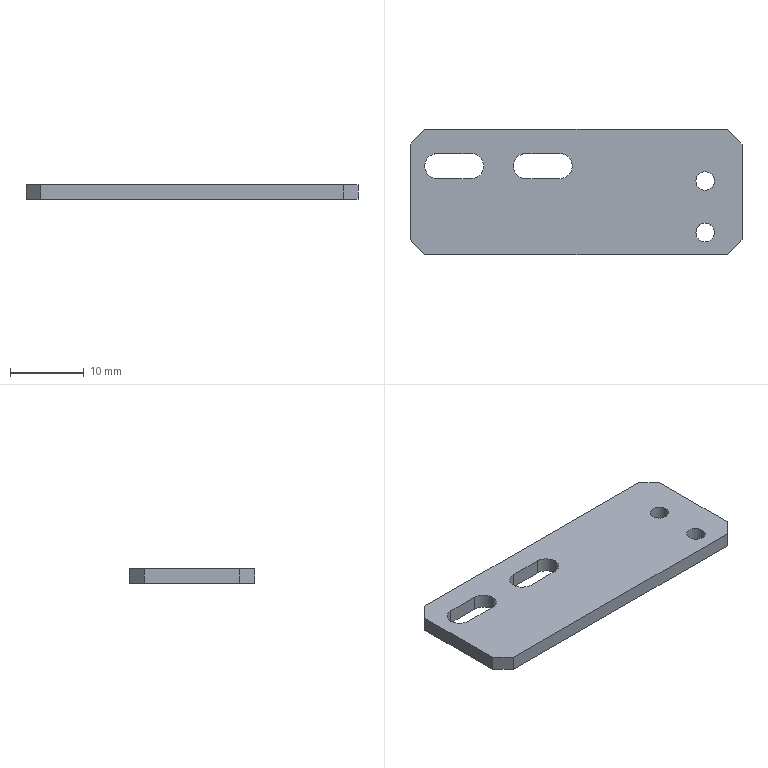Part | STEP file | FBDS-CS-006 | 1 solid | 24 faces | box 45 x 17 x 2 mm | volume 1395 mm3 | plane 14 | cylinder 10 | commonest cylinder face diameters 3.4 x6 2.5 x4
STEP:
#1=CARTESIAN_POINT('',(16.25,1.5,-2.));
#2=VERTEX_POINT('',#1);
#3=CARTESIAN_POINT('',(18.75,1.5,-2.));
#4=VERTEX_POINT('',#3);
#5=CARTESIAN_POINT('',(17.5,1.5,-2.));
#6=DIRECTION('',(0.,0.,1.));
#7=DIRECTION('',(1.,0.,0.));
#8=AXIS2_PLACEMENT_3D('',#5,#6,#7);
#9=CIRCLE('',#8,1.25);
#10=EDGE_CURVE('',#2,#4,#9,.T.);
#11=ORIENTED_EDGE('',*,*,#10,.F.);
#12=CARTESIAN_POINT('',(16.25,1.5,0.));
#13=VERTEX_POINT('',#12);
#14=CARTESIAN_POINT('',(16.25,1.5,0.));
#15=DIRECTION('',(0.,0.,1.));
#16=VECTOR('',#15,1000.);
#17=LINE('',#14,#16);
#18=EDGE_CURVE('',#2,#13,#17,.T.);
#19=ORIENTED_EDGE('',*,*,#18,.T.);
#20=CARTESIAN_POINT('',(18.75,1.5,0.));
#21=VERTEX_POINT('',#20);
#22=CARTESIAN_POINT('',(17.5,1.5,0.));
#23=DIRECTION('',(0.,0.,1.));
#24=DIRECTION('',(1.,0.,0.));
#25=AXIS2_PLACEMENT_3D('',#22,#23,#24);
#26=CIRCLE('',#25,1.25);
#27=EDGE_CURVE('',#13,#21,#26,.T.);
#28=ORIENTED_EDGE('',*,*,#27,.T.);
#29=CARTESIAN_POINT('',(18.75,1.5,0.));
#30=DIRECTION('',(0.,0.,1.));
#31=VECTOR('',#30,1000.);
#32=LINE('',#29,#31);
#33=EDGE_CURVE('',#4,#21,#32,.T.);
#34=ORIENTED_EDGE('',*,*,#33,.F.);
#35=EDGE_LOOP('',(#11,#19,#28,#34));
#36=FACE_OUTER_BOUND('',#35,.T.);
#37=CARTESIAN_POINT('',(17.5,1.5,0.));
#38=DIRECTION('',(0.,0.,1.));
#39=DIRECTION('',(1.,0.,0.));
#40=AXIS2_PLACEMENT_3D('',#37,#38,#39);
#41=CYLINDRICAL_SURFACE('',#40,1.25);
#42=ADVANCED_FACE('',(#36),#41,.F.);
#43=CARTESIAN_POINT('',(16.25,-5.5,-2.));
#44=VERTEX_POINT('',#43);
#45=CARTESIAN_POINT('',(18.75,-5.5,-2.));
#46=VERTEX_POINT('',#45);
#47=CARTESIAN_POINT('',(17.5,-5.5,-2.));
#48=DIRECTION('',(0.,0.,1.));
#49=DIRECTION('',(1.,0.,0.));
#50=AXIS2_PLACEMENT_3D('',#47,#48,#49);
#51=CIRCLE('',#50,1.25);
#52=EDGE_CURVE('',#44,#46,#51,.T.);
#53=ORIENTED_EDGE('',*,*,#52,.F.);
#54=CARTESIAN_POINT('',(16.25,-5.5,0.));
#55=VERTEX_POINT('',#54);
#56=CARTESIAN_POINT('',(16.25,-5.5,0.));
#57=DIRECTION('',(0.,0.,1.));
#58=VECTOR('',#57,1000.);
#59=LINE('',#56,#58);
#60=EDGE_CURVE('',#44,#55,#59,.T.);
#61=ORIENTED_EDGE('',*,*,#60,.T.);
#62=CARTESIAN_POINT('',(18.75,-5.5,0.));
#63=VERTEX_POINT('',#62);
#64=CARTESIAN_POINT('',(17.5,-5.5,0.));
#65=DIRECTION('',(0.,0.,1.));
#66=DIRECTION('',(1.,0.,0.));
#67=AXIS2_PLACEMENT_3D('',#64,#65,#66);
#68=CIRCLE('',#67,1.25);
#69=EDGE_CURVE('',#55,#63,#68,.T.);
#70=ORIENTED_EDGE('',*,*,#69,.T.);
#71=CARTESIAN_POINT('',(18.75,-5.5,0.));
#72=DIRECTION('',(0.,0.,1.));
#73=VECTOR('',#72,1000.);
#74=LINE('',#71,#73);
#75=EDGE_CURVE('',#46,#63,#74,.T.);
#76=ORIENTED_EDGE('',*,*,#75,.F.);
#77=EDGE_LOOP('',(#53,#61,#70,#76));
#78=FACE_OUTER_BOUND('',#77,.T.);
#79=CARTESIAN_POINT('',(17.5,-5.5,0.));
#80=DIRECTION('',(0.,0.,1.));
#81=DIRECTION('',(1.,0.,0.));
#82=AXIS2_PLACEMENT_3D('',#79,#80,#81);
#83=CYLINDRICAL_SURFACE('',#82,1.25);
#84=ADVANCED_FACE('',(#78),#83,.F.);
#85=CARTESIAN_POINT('',(-12.5,3.5,-2.));
#86=VERTEX_POINT('',#85);
#87=CARTESIAN_POINT('',(-14.2,5.2,-2.));
#88=VERTEX_POINT('',#87);
#89=CARTESIAN_POINT('',(-14.2,3.5,-2.));
#90=DIRECTION('',(0.,0.,1.));
#91=DIRECTION('',(1.,0.,0.));
#92=AXIS2_PLACEMENT_3D('',#89,#90,#91);
#93=CIRCLE('',#92,1.7);
#94=EDGE_CURVE('',#86,#88,#93,.T.);
#95=ORIENTED_EDGE('',*,*,#94,.F.);
#96=CARTESIAN_POINT('',(-12.5,3.5,0.));
#97=VERTEX_POINT('',#96);
#98=CARTESIAN_POINT('',(-12.5,3.5,0.));
#99=DIRECTION('',(0.,0.,1.));
#100=VECTOR('',#99,1000.);
#101=LINE('',#98,#100);
#102=EDGE_CURVE('',#86,#97,#101,.T.);
#103=ORIENTED_EDGE('',*,*,#102,.T.);
#104=CARTESIAN_POINT('',(-14.2,5.2,0.));
#105=VERTEX_POINT('',#104);
#106=CARTESIAN_POINT('',(-14.2,3.5,0.));
#107=DIRECTION('',(0.,0.,1.));
#108=DIRECTION('',(1.,0.,0.));
#109=AXIS2_PLACEMENT_3D('',#106,#107,#108);
#110=CIRCLE('',#109,1.7);
#111=EDGE_CURVE('',#97,#105,#110,.T.);
#112=ORIENTED_EDGE('',*,*,#111,.T.);
#113=CARTESIAN_POINT('',(-14.2,5.2,0.));
#114=DIRECTION('',(0.,0.,1.));
#115=VECTOR('',#114,1000.);
#116=LINE('',#113,#115);
#117=EDGE_CURVE('',#88,#105,#116,.T.);
#118=ORIENTED_EDGE('',*,*,#117,.F.);
#119=EDGE_LOOP('',(#95,#103,#112,#118));
#120=FACE_OUTER_BOUND('',#119,.T.);
#121=CARTESIAN_POINT('',(-14.2,3.5,0.));
#122=DIRECTION('',(0.,0.,1.));
#123=DIRECTION('',(1.,0.,0.));
#124=AXIS2_PLACEMENT_3D('',#121,#122,#123);
#125=CYLINDRICAL_SURFACE('',#124,1.7);
#126=ADVANCED_FACE('',(#120),#125,.F.);
#127=CARTESIAN_POINT('',(-0.5,3.5,-2.));
#128=VERTEX_POINT('',#127);
#129=CARTESIAN_POINT('',(-2.2,5.2,-2.));
#130=VERTEX_POINT('',#129);
#131=CARTESIAN_POINT('',(-2.2,3.5,-2.));
#132=DIRECTION('',(0.,0.,1.));
#133=DIRECTION('',(1.,0.,0.));
#134=AXIS2_PLACEMENT_3D('',#131,#132,#133);
#135=CIRCLE('',#134,1.7);
#136=EDGE_CURVE('',#128,#130,#135,.T.);
#137=ORIENTED_EDGE('',*,*,#136,.F.);
#138=CARTESIAN_POINT('',(-0.5,3.5,0.));
#139=VERTEX_POINT('',#138);
#140=CARTESIAN_POINT('',(-0.5,3.5,0.));
#141=DIRECTION('',(0.,0.,1.));
#142=VECTOR('',#141,1000.);
#143=LINE('',#140,#142);
#144=EDGE_CURVE('',#128,#139,#143,.T.);
#145=ORIENTED_EDGE('',*,*,#144,.T.);
#146=CARTESIAN_POINT('',(-2.2,5.2,0.));
#147=VERTEX_POINT('',#146);
#148=CARTESIAN_POINT('',(-2.2,3.5,0.));
#149=DIRECTION('',(0.,0.,1.));
#150=DIRECTION('',(1.,0.,0.));
#151=AXIS2_PLACEMENT_3D('',#148,#149,#150);
#152=CIRCLE('',#151,1.7);
#153=EDGE_CURVE('',#139,#147,#152,.T.);
#154=ORIENTED_EDGE('',*,*,#153,.T.);
#155=CARTESIAN_POINT('',(-2.2,5.2,0.));
#156=DIRECTION('',(0.,0.,1.));
#157=VECTOR('',#156,1000.);
#158=LINE('',#155,#157);
#159=EDGE_CURVE('',#130,#147,#158,.T.);
#160=ORIENTED_EDGE('',*,*,#159,.F.);
#161=EDGE_LOOP('',(#137,#145,#154,#160));
#162=FACE_OUTER_BOUND('',#161,.T.);
#163=CARTESIAN_POINT('',(-2.2,3.5,0.));
#164=DIRECTION('',(0.,0.,1.));
#165=DIRECTION('',(1.,0.,0.));
#166=AXIS2_PLACEMENT_3D('',#163,#164,#165);
#167=CYLINDRICAL_SURFACE('',#166,1.7);
#168=ADVANCED_FACE('',(#162),#167,.F.);
#169=CARTESIAN_POINT('',(22.5,-6.5,-2.));
#170=VERTEX_POINT('',#169);
#171=CARTESIAN_POINT('',(22.5,6.5,-2.));
#172=VERTEX_POINT('',#171);
#173=CARTESIAN_POINT('',(22.5,8.5,-2.));
#174=DIRECTION('',(0.,1.,0.));
#175=VECTOR('',#174,1000.);
#176=LINE('',#173,#175);
#177=EDGE_CURVE('',#170,#172,#176,.T.);
#178=ORIENTED_EDGE('',*,*,#177,.T.);
#179=CARTESIAN_POINT('',(22.5,6.5,0.));
#180=VERTEX_POINT('',#179);
#181=CARTESIAN_POINT('',(22.5,6.5,-2.));
#182=DIRECTION('',(0.,0.,1.));
#183=VECTOR('',#182,1000.);
#184=LINE('',#181,#183);
#185=EDGE_CURVE('',#172,#180,#184,.T.);
#186=ORIENTED_EDGE('',*,*,#185,.T.);
#187=CARTESIAN_POINT('',(22.5,-6.5,0.));
#188=VERTEX_POINT('',#187);
#189=CARTESIAN_POINT('',(22.5,8.5,0.));
#190=DIRECTION('',(0.,1.,0.));
#191=VECTOR('',#190,1000.);
#192=LINE('',#189,#191);
#193=EDGE_CURVE('',#188,#180,#192,.T.);
#194=ORIENTED_EDGE('',*,*,#193,.F.);
#195=CARTESIAN_POINT('',(22.5,-6.5,-2.));
#196=DIRECTION('',(0.,0.,-1.));
#197=VECTOR('',#196,1000.);
#198=LINE('',#195,#197);
#199=EDGE_CURVE('',#188,#170,#198,.T.);
#200=ORIENTED_EDGE('',*,*,#199,.T.);
#201=EDGE_LOOP('',(#178,#186,#194,#200));
#202=FACE_OUTER_BOUND('',#201,.T.);
#203=CARTESIAN_POINT('',(22.5,8.5,-2.));
#204=DIRECTION('',(1.,0.,0.));
#205=DIRECTION('',(0.,0.,-1.));
#206=AXIS2_PLACEMENT_3D('',#203,#204,#205);
#207=PLANE('',#206);
#208=ADVANCED_FACE('',(#202),#207,.T.);
#209=CARTESIAN_POINT('',(-20.5,-8.5,-2.));
#210=VERTEX_POINT('',#209);
#211=CARTESIAN_POINT('',(20.5,-8.5,-2.));
#212=VERTEX_POINT('',#211);
#213=CARTESIAN_POINT('',(-22.5,-8.5,-2.));
#214=DIRECTION('',(1.,0.,0.));
#215=VECTOR('',#214,1000.);
#216=LINE('',#213,#215);
#217=EDGE_CURVE('',#210,#212,#216,.T.);
#218=ORIENTED_EDGE('',*,*,#217,.T.);
#219=CARTESIAN_POINT('',(20.5,-8.5,0.));
#220=VERTEX_POINT('',#219);
#221=CARTESIAN_POINT('',(20.5,-8.5,-2.));
#222=DIRECTION('',(0.,0.,1.));
#223=VECTOR('',#222,1000.);
#224=LINE('',#221,#223);
#225=EDGE_CURVE('',#212,#220,#224,.T.);
#226=ORIENTED_EDGE('',*,*,#225,.T.);
#227=CARTESIAN_POINT('',(-20.5,-8.5,0.));
#228=VERTEX_POINT('',#227);
#229=CARTESIAN_POINT('',(-22.5,-8.5,0.));
#230=DIRECTION('',(1.,0.,0.));
#231=VECTOR('',#230,1000.);
#232=LINE('',#229,#231);
#233=EDGE_CURVE('',#228,#220,#232,.T.);
#234=ORIENTED_EDGE('',*,*,#233,.F.);
#235=CARTESIAN_POINT('',(-20.5,-8.5,-2.));
#236=DIRECTION('',(0.,0.,-1.));
#237=VECTOR('',#236,1000.);
#238=LINE('',#235,#237);
#239=EDGE_CURVE('',#228,#210,#238,.T.);
#240=ORIENTED_EDGE('',*,*,#239,.T.);
#241=EDGE_LOOP('',(#218,#226,#234,#240));
#242=FACE_OUTER_BOUND('',#241,.T.);
#243=CARTESIAN_POINT('',(-22.5,-8.5,-2.));
#244=DIRECTION('',(0.,-1.,0.));
#245=DIRECTION('',(0.,0.,-1.));
#246=AXIS2_PLACEMENT_3D('',#243,#244,#245);
#247=PLANE('',#246);
#248=ADVANCED_FACE('',(#242),#247,.T.);
#249=CARTESIAN_POINT('',(-22.5,6.5,-2.));
#250=VERTEX_POINT('',#249);
#251=CARTESIAN_POINT('',(-22.5,-6.5,-2.));
#252=VERTEX_POINT('',#251);
#253=CARTESIAN_POINT('',(-22.5,8.5,-2.));
#254=DIRECTION('',(0.,-1.,0.));
#255=VECTOR('',#254,1000.);
#256=LINE('',#253,#255);
#257=EDGE_CURVE('',#250,#252,#256,.T.);
#258=ORIENTED_EDGE('',*,*,#257,.T.);
#259=CARTESIAN_POINT('',(-22.5,-6.5,0.));
#260=VERTEX_POINT('',#259);
#261=CARTESIAN_POINT('',(-22.5,-6.5,-2.));
#262=DIRECTION('',(0.,0.,1.));
#263=VECTOR('',#262,1000.);
#264=LINE('',#261,#263);
#265=EDGE_CURVE('',#252,#260,#264,.T.);
#266=ORIENTED_EDGE('',*,*,#265,.T.);
#267=CARTESIAN_POINT('',(-22.5,6.5,0.));
#268=VERTEX_POINT('',#267);
#269=CARTESIAN_POINT('',(-22.5,8.5,0.));
#270=DIRECTION('',(0.,-1.,0.));
#271=VECTOR('',#270,1000.);
#272=LINE('',#269,#271);
#273=EDGE_CURVE('',#268,#260,#272,.T.);
#274=ORIENTED_EDGE('',*,*,#273,.F.);
#275=CARTESIAN_POINT('',(-22.5,6.5,-2.));
#276=DIRECTION('',(0.,0.,-1.));
#277=VECTOR('',#276,1000.);
#278=LINE('',#275,#277);
#279=EDGE_CURVE('',#268,#250,#278,.T.);
#280=ORIENTED_EDGE('',*,*,#279,.T.);
#281=EDGE_LOOP('',(#258,#266,#274,#280));
#282=FACE_OUTER_BOUND('',#281,.T.);
#283=CARTESIAN_POINT('',(-22.5,8.5,-2.));
#284=DIRECTION('',(-1.,0.,0.));
#285=DIRECTION('',(0.,-1.,0.));
#286=AXIS2_PLACEMENT_3D('',#283,#284,#285);
#287=PLANE('',#286);
#288=ADVANCED_FACE('',(#282),#287,.T.);
#289=CARTESIAN_POINT('',(20.5,8.5,0.));
#290=VERTEX_POINT('',#289);
#291=CARTESIAN_POINT('',(-20.5,8.5,0.));
#292=VERTEX_POINT('',#291);
#293=CARTESIAN_POINT('',(-22.5,8.5,0.));
#294=DIRECTION('',(-1.,0.,0.));
#295=VECTOR('',#294,1000.);
#296=LINE('',#293,#295);
#297=EDGE_CURVE('',#290,#292,#296,.T.);
#298=ORIENTED_EDGE('',*,*,#297,.F.);
#299=CARTESIAN_POINT('',(20.5,8.5,-2.));
#300=VERTEX_POINT('',#299);
#301=CARTESIAN_POINT('',(20.5,8.5,-2.));
#302=DIRECTION('',(0.,0.,-1.));
#303=VECTOR('',#302,1000.);
#304=LINE('',#301,#303);
#305=EDGE_CURVE('',#290,#300,#304,.T.);
#306=ORIENTED_EDGE('',*,*,#305,.T.);
#307=CARTESIAN_POINT('',(-20.5,8.5,-2.));
#308=VERTEX_POINT('',#307);
#309=CARTESIAN_POINT('',(-22.5,8.5,-2.));
#310=DIRECTION('',(-1.,0.,0.));
#311=VECTOR('',#310,1000.);
#312=LINE('',#309,#311);
#313=EDGE_CURVE('',#300,#308,#312,.T.);
#314=ORIENTED_EDGE('',*,*,#313,.T.);
#315=CARTESIAN_POINT('',(-20.5,8.5,-2.));
#316=DIRECTION('',(0.,0.,1.));
#317=VECTOR('',#316,1000.);
#318=LINE('',#315,#317);
#319=EDGE_CURVE('',#308,#292,#318,.T.);
#320=ORIENTED_EDGE('',*,*,#319,.T.);
#321=EDGE_LOOP('',(#298,#306,#314,#320));
#322=FACE_OUTER_BOUND('',#321,.T.);
#323=CARTESIAN_POINT('',(-22.5,8.5,-2.));
#324=DIRECTION('',(0.,1.,0.));
#325=DIRECTION('',(0.,0.,1.));
#326=AXIS2_PLACEMENT_3D('',#323,#324,#325);
#327=PLANE('',#326);
#328=ADVANCED_FACE('',(#322),#327,.T.);
#329=CARTESIAN_POINT('',(17.5,1.5,-2.));
#330=DIRECTION('',(0.,0.,1.));
#331=DIRECTION('',(1.,0.,0.));
#332=AXIS2_PLACEMENT_3D('',#329,#330,#331);
#333=CIRCLE('',#332,1.25);
#334=EDGE_CURVE('',#4,#2,#333,.T.);
#335=ORIENTED_EDGE('',*,*,#334,.T.);
#336=ORIENTED_EDGE('',*,*,#10,.T.);
#337=EDGE_LOOP('',(#335,#336));
#338=FACE_BOUND('',#337,.T.);
#339=CARTESIAN_POINT('',(17.5,-5.5,-2.));
#340=DIRECTION('',(0.,0.,1.));
#341=DIRECTION('',(1.,0.,0.));
#342=AXIS2_PLACEMENT_3D('',#339,#340,#341);
#343=CIRCLE('',#342,1.25);
#344=EDGE_CURVE('',#46,#44,#343,.T.);
#345=ORIENTED_EDGE('',*,*,#344,.T.);
#346=ORIENTED_EDGE('',*,*,#52,.T.);
#347=EDGE_LOOP('',(#345,#346));
#348=FACE_BOUND('',#347,.T.);
#349=CARTESIAN_POINT('',(-14.2,1.8,-2.));
#350=VERTEX_POINT('',#349);
#351=CARTESIAN_POINT('',(-14.2,3.5,-2.));
#352=DIRECTION('',(0.,0.,1.));
#353=DIRECTION('',(1.,0.,0.));
#354=AXIS2_PLACEMENT_3D('',#351,#352,#353);
#355=CIRCLE('',#354,1.7);
#356=EDGE_CURVE('',#350,#86,#355,.T.);
#357=ORIENTED_EDGE('',*,*,#356,.T.);
#358=ORIENTED_EDGE('',*,*,#94,.T.);
#359=CARTESIAN_POINT('',(-18.8,5.2,-2.));
#360=VERTEX_POINT('',#359);
#361=CARTESIAN_POINT('',(0.,5.2,-2.));
#362=DIRECTION('',(-1.,0.,0.));
#363=VECTOR('',#362,1000.);
#364=LINE('',#361,#363);
#365=EDGE_CURVE('',#88,#360,#364,.T.);
#366=ORIENTED_EDGE('',*,*,#365,.T.);
#367=CARTESIAN_POINT('',(-18.8,1.8,-2.));
#368=VERTEX_POINT('',#367);
#369=CARTESIAN_POINT('',(-18.8,3.5,-2.));
#370=DIRECTION('',(0.,0.,1.));
#371=DIRECTION('',(1.,0.,0.));
#372=AXIS2_PLACEMENT_3D('',#369,#370,#371);
#373=CIRCLE('',#372,1.7);
#374=EDGE_CURVE('',#360,#368,#373,.T.);
#375=ORIENTED_EDGE('',*,*,#374,.T.);
#376=CARTESIAN_POINT('',(0.,1.8,-2.));
#377=DIRECTION('',(1.,0.,0.));
#378=VECTOR('',#377,1000.);
#379=LINE('',#376,#378);
#380=EDGE_CURVE('',#368,#350,#379,.T.);
#381=ORIENTED_EDGE('',*,*,#380,.T.);
#382=EDGE_LOOP('',(#357,#358,#366,#375,#381));
#383=FACE_BOUND('',#382,.T.);
#384=CARTESIAN_POINT('',(-6.8,1.8,-2.));
#385=VERTEX_POINT('',#384);
#386=CARTESIAN_POINT('',(-2.2,1.8,-2.));
#387=VERTEX_POINT('',#386);
#388=CARTESIAN_POINT('',(0.,1.8,-2.));
#389=DIRECTION('',(1.,0.,0.));
#390=VECTOR('',#389,1000.);
#391=LINE('',#388,#390);
#392=EDGE_CURVE('',#385,#387,#391,.T.);
#393=ORIENTED_EDGE('',*,*,#392,.T.);
#394=CARTESIAN_POINT('',(-2.2,3.5,-2.));
#395=DIRECTION('',(0.,0.,1.));
#396=DIRECTION('',(1.,0.,0.));
#397=AXIS2_PLACEMENT_3D('',#394,#395,#396);
#398=CIRCLE('',#397,1.7);
#399=EDGE_CURVE('',#387,#128,#398,.T.);
#400=ORIENTED_EDGE('',*,*,#399,.T.);
#401=ORIENTED_EDGE('',*,*,#136,.T.);
#402=CARTESIAN_POINT('',(-6.8,5.2,-2.));
#403=VERTEX_POINT('',#402);
#404=CARTESIAN_POINT('',(0.,5.2,-2.));
#405=DIRECTION('',(-1.,0.,0.));
#406=VECTOR('',#405,1000.);
#407=LINE('',#404,#406);
#408=EDGE_CURVE('',#130,#403,#407,.T.);
#409=ORIENTED_EDGE('',*,*,#408,.T.);
#410=CARTESIAN_POINT('',(-6.8,3.5,-2.));
#411=DIRECTION('',(0.,0.,1.));
#412=DIRECTION('',(1.,0.,0.));
#413=AXIS2_PLACEMENT_3D('',#410,#411,#412);
#414=CIRCLE('',#413,1.7);
#415=EDGE_CURVE('',#403,#385,#414,.T.);
#416=ORIENTED_EDGE('',*,*,#415,.T.);
#417=EDGE_LOOP('',(#393,#400,#401,#409,#416));
#418=FACE_BOUND('',#417,.T.);
#419=ORIENTED_EDGE('',*,*,#313,.F.);
#420=CARTESIAN_POINT('',(22.5,6.5,-2.));
#421=DIRECTION('',(0.7071,-0.7071,0.));
#422=VECTOR('',#421,1000.);
#423=LINE('',#420,#422);
#424=EDGE_CURVE('',#300,#172,#423,.T.);
#425=ORIENTED_EDGE('',*,*,#424,.T.);
#426=ORIENTED_EDGE('',*,*,#177,.F.);
#427=CARTESIAN_POINT('',(20.5,-8.5,-2.));
#428=DIRECTION('',(-0.7071,-0.7071,0.));
#429=VECTOR('',#428,1000.);
#430=LINE('',#427,#429);
#431=EDGE_CURVE('',#170,#212,#430,.T.);
#432=ORIENTED_EDGE('',*,*,#431,.T.);
#433=ORIENTED_EDGE('',*,*,#217,.F.);
#434=CARTESIAN_POINT('',(-22.5,-6.5,-2.));
#435=DIRECTION('',(-0.7071,0.7071,0.));
#436=VECTOR('',#435,1000.);
#437=LINE('',#434,#436);
#438=EDGE_CURVE('',#210,#252,#437,.T.);
#439=ORIENTED_EDGE('',*,*,#438,.T.);
#440=ORIENTED_EDGE('',*,*,#257,.F.);
#441=CARTESIAN_POINT('',(-20.5,8.5,-2.));
#442=DIRECTION('',(0.7071,0.7071,0.));
#443=VECTOR('',#442,1000.);
#444=LINE('',#441,#443);
#445=EDGE_CURVE('',#250,#308,#444,.T.);
#446=ORIENTED_EDGE('',*,*,#445,.T.);
#447=EDGE_LOOP('',(#419,#425,#426,#432,#433,#439,#440,#446));
#448=FACE_OUTER_BOUND('',#447,.T.);
#449=CARTESIAN_POINT('',(0.,0.,-2.));
#450=DIRECTION('',(0.,0.,1.));
#451=DIRECTION('',(1.,0.,0.));
#452=AXIS2_PLACEMENT_3D('',#449,#450,#451);
#453=PLANE('',#452);
#454=ADVANCED_FACE('',(#338,#348,#383,#418,#448),#453,.F.);
#455=CARTESIAN_POINT('',(17.5,1.5,0.));
#456=DIRECTION('',(0.,0.,1.));
#457=DIRECTION('',(1.,0.,0.));
#458=AXIS2_PLACEMENT_3D('',#455,#456,#457);
#459=CIRCLE('',#458,1.25);
#460=EDGE_CURVE('',#21,#13,#459,.T.);
#461=ORIENTED_EDGE('',*,*,#460,.F.);
#462=ORIENTED_EDGE('',*,*,#27,.F.);
#463=EDGE_LOOP('',(#461,#462));
#464=FACE_BOUND('',#463,.T.);
#465=CARTESIAN_POINT('',(17.5,-5.5,0.));
#466=DIRECTION('',(0.,0.,1.));
#467=DIRECTION('',(1.,0.,0.));
#468=AXIS2_PLACEMENT_3D('',#465,#466,#467);
#469=CIRCLE('',#468,1.25);
#470=EDGE_CURVE('',#63,#55,#469,.T.);
#471=ORIENTED_EDGE('',*,*,#470,.F.);
#472=ORIENTED_EDGE('',*,*,#69,.F.);
#473=EDGE_LOOP('',(#471,#472));
#474=FACE_BOUND('',#473,.T.);
#475=CARTESIAN_POINT('',(-18.8,1.8,0.));
#476=VERTEX_POINT('',#475);
#477=CARTESIAN_POINT('',(-14.2,1.8,0.));
#478=VERTEX_POINT('',#477);
#479=CARTESIAN_POINT('',(-18.8,1.8,0.));
#480=DIRECTION('',(1.,0.,0.));
#481=VECTOR('',#480,1000.);
#482=LINE('',#479,#481);
#483=EDGE_CURVE('',#476,#478,#482,.T.);
#484=ORIENTED_EDGE('',*,*,#483,.F.);
#485=CARTESIAN_POINT('',(-18.8,5.2,0.));
#486=VERTEX_POINT('',#485);
#487=CARTESIAN_POINT('',(-18.8,3.5,0.));
#488=DIRECTION('',(0.,0.,1.));
#489=DIRECTION('',(1.,0.,0.));
#490=AXIS2_PLACEMENT_3D('',#487,#488,#489);
#491=CIRCLE('',#490,1.7);
#492=EDGE_CURVE('',#486,#476,#491,.T.);
#493=ORIENTED_EDGE('',*,*,#492,.F.);
#494=CARTESIAN_POINT('',(-18.8,5.2,0.));
#495=DIRECTION('',(1.,0.,0.));
#496=VECTOR('',#495,1000.);
#497=LINE('',#494,#496);
#498=EDGE_CURVE('',#486,#105,#497,.T.);
#499=ORIENTED_EDGE('',*,*,#498,.T.);
#500=ORIENTED_EDGE('',*,*,#111,.F.);
#501=CARTESIAN_POINT('',(-14.2,3.5,0.));
#502=DIRECTION('',(0.,0.,1.));
#503=DIRECTION('',(1.,0.,0.));
#504=AXIS2_PLACEMENT_3D('',#501,#502,#503);
#505=CIRCLE('',#504,1.7);
#506=EDGE_CURVE('',#478,#97,#505,.T.);
#507=ORIENTED_EDGE('',*,*,#506,.F.);
#508=EDGE_LOOP('',(#484,#493,#499,#500,#507));
#509=FACE_BOUND('',#508,.T.);
#510=CARTESIAN_POINT('',(-6.8,1.8,0.));
#511=VERTEX_POINT('',#510);
#512=CARTESIAN_POINT('',(-2.2,1.8,0.));
#513=VERTEX_POINT('',#512);
#514=CARTESIAN_POINT('',(-6.8,1.8,0.));
#515=DIRECTION('',(1.,0.,0.));
#516=VECTOR('',#515,1000.);
#517=LINE('',#514,#516);
#518=EDGE_CURVE('',#511,#513,#517,.T.);
#519=ORIENTED_EDGE('',*,*,#518,.F.);
#520=CARTESIAN_POINT('',(-6.8,5.2,0.));
#521=VERTEX_POINT('',#520);
#522=CARTESIAN_POINT('',(-6.8,3.5,0.));
#523=DIRECTION('',(0.,0.,1.));
#524=DIRECTION('',(1.,0.,0.));
#525=AXIS2_PLACEMENT_3D('',#522,#523,#524);
#526=CIRCLE('',#525,1.7);
#527=EDGE_CURVE('',#521,#511,#526,.T.);
#528=ORIENTED_EDGE('',*,*,#527,.F.);
#529=CARTESIAN_POINT('',(-6.8,5.2,0.));
#530=DIRECTION('',(1.,0.,0.));
#531=VECTOR('',#530,1000.);
#532=LINE('',#529,#531);
#533=EDGE_CURVE('',#521,#147,#532,.T.);
#534=ORIENTED_EDGE('',*,*,#533,.T.);
#535=ORIENTED_EDGE('',*,*,#153,.F.);
#536=CARTESIAN_POINT('',(-2.2,3.5,0.));
#537=DIRECTION('',(0.,0.,1.));
#538=DIRECTION('',(1.,0.,0.));
#539=AXIS2_PLACEMENT_3D('',#536,#537,#538);
#540=CIRCLE('',#539,1.7);
#541=EDGE_CURVE('',#513,#139,#540,.T.);
#542=ORIENTED_EDGE('',*,*,#541,.F.);
#543=EDGE_LOOP('',(#519,#528,#534,#535,#542));
#544=FACE_BOUND('',#543,.T.);
#545=ORIENTED_EDGE('',*,*,#193,.T.);
#546=CARTESIAN_POINT('',(14.5,14.5,0.));
#547=DIRECTION('',(-0.7071,0.7071,0.));
#548=VECTOR('',#547,1000.);
#549=LINE('',#546,#548);
#550=EDGE_CURVE('',#180,#290,#549,.T.);
#551=ORIENTED_EDGE('',*,*,#550,.T.);
#552=ORIENTED_EDGE('',*,*,#297,.T.);
#553=CARTESIAN_POINT('',(-14.5,14.5,0.));
#554=DIRECTION('',(-0.7071,-0.7071,0.));
#555=VECTOR('',#554,1000.);
#556=LINE('',#553,#555);
#557=EDGE_CURVE('',#292,#268,#556,.T.);
#558=ORIENTED_EDGE('',*,*,#557,.T.);
#559=ORIENTED_EDGE('',*,*,#273,.T.);
#560=CARTESIAN_POINT('',(-14.5,-14.5,0.));
#561=DIRECTION('',(0.7071,-0.7071,0.));
#562=VECTOR('',#561,1000.);
#563=LINE('',#560,#562);
#564=EDGE_CURVE('',#260,#228,#563,.T.);
#565=ORIENTED_EDGE('',*,*,#564,.T.);
#566=ORIENTED_EDGE('',*,*,#233,.T.);
#567=CARTESIAN_POINT('',(14.5,-14.5,0.));
#568=DIRECTION('',(0.7071,0.7071,0.));
#569=VECTOR('',#568,1000.);
#570=LINE('',#567,#569);
#571=EDGE_CURVE('',#220,#188,#570,.T.);
#572=ORIENTED_EDGE('',*,*,#571,.T.);
#573=EDGE_LOOP('',(#545,#551,#552,#558,#559,#565,#566,#572));
#574=FACE_OUTER_BOUND('',#573,.T.);
#575=CARTESIAN_POINT('',(0.,0.,0.));
#576=DIRECTION('',(0.,0.,1.));
#577=DIRECTION('',(1.,0.,0.));
#578=AXIS2_PLACEMENT_3D('',#575,#576,#577);
#579=PLANE('',#578);
#580=ADVANCED_FACE('',(#464,#474,#509,#544,#574),#579,.T.);
#581=CARTESIAN_POINT('',(-6.8,1.8,0.));
#582=DIRECTION('',(0.,0.,1.));
#583=VECTOR('',#582,1000.);
#584=LINE('',#581,#583);
#585=EDGE_CURVE('',#385,#511,#584,.T.);
#586=ORIENTED_EDGE('',*,*,#585,.T.);
#587=ORIENTED_EDGE('',*,*,#518,.T.);
#588=CARTESIAN_POINT('',(-2.2,1.8,0.));
#589=DIRECTION('',(0.,0.,-1.));
#590=VECTOR('',#589,1000.);
#591=LINE('',#588,#590);
#592=EDGE_CURVE('',#513,#387,#591,.T.);
#593=ORIENTED_EDGE('',*,*,#592,.T.);
#594=ORIENTED_EDGE('',*,*,#392,.F.);
#595=EDGE_LOOP('',(#586,#587,#593,#594));
#596=FACE_OUTER_BOUND('',#595,.T.);
#597=CARTESIAN_POINT('',(-6.8,1.8,0.));
#598=DIRECTION('',(0.,-1.,0.));
#599=DIRECTION('',(1.,0.,0.));
#600=AXIS2_PLACEMENT_3D('',#597,#598,#599);
#601=PLANE('',#600);
#602=ADVANCED_FACE('',(#596),#601,.F.);
#603=ORIENTED_EDGE('',*,*,#159,.T.);
#604=ORIENTED_EDGE('',*,*,#533,.F.);
#605=CARTESIAN_POINT('',(-6.8,5.2,0.));
#606=DIRECTION('',(0.,0.,-1.));
#607=VECTOR('',#606,1000.);
#608=LINE('',#605,#607);
#609=EDGE_CURVE('',#521,#403,#608,.T.);
#610=ORIENTED_EDGE('',*,*,#609,.T.);
#611=ORIENTED_EDGE('',*,*,#408,.F.);
#612=EDGE_LOOP('',(#603,#604,#610,#611));
#613=FACE_OUTER_BOUND('',#612,.T.);
#614=CARTESIAN_POINT('',(-6.8,5.2,0.));
#615=DIRECTION('',(0.,1.,0.));
#616=DIRECTION('',(-1.,0.,0.));
#617=AXIS2_PLACEMENT_3D('',#614,#615,#616);
#618=PLANE('',#617);
#619=ADVANCED_FACE('',(#613),#618,.F.);
#620=ORIENTED_EDGE('',*,*,#144,.F.);
#621=ORIENTED_EDGE('',*,*,#399,.F.);
#622=ORIENTED_EDGE('',*,*,#592,.F.);
#623=ORIENTED_EDGE('',*,*,#541,.T.);
#624=EDGE_LOOP('',(#620,#621,#622,#623));
#625=FACE_OUTER_BOUND('',#624,.T.);
#626=CARTESIAN_POINT('',(-2.2,3.5,0.));
#627=DIRECTION('',(0.,0.,1.));
#628=DIRECTION('',(1.,0.,0.));
#629=AXIS2_PLACEMENT_3D('',#626,#627,#628);
#630=CYLINDRICAL_SURFACE('',#629,1.7);
#631=ADVANCED_FACE('',(#625),#630,.F.);
#632=ORIENTED_EDGE('',*,*,#609,.F.);
#633=ORIENTED_EDGE('',*,*,#527,.T.);
#634=ORIENTED_EDGE('',*,*,#585,.F.);
#635=ORIENTED_EDGE('',*,*,#415,.F.);
#636=EDGE_LOOP('',(#632,#633,#634,#635));
#637=FACE_OUTER_BOUND('',#636,.T.);
#638=CARTESIAN_POINT('',(-6.8,3.5,0.));
#639=DIRECTION('',(0.,0.,1.));
#640=DIRECTION('',(1.,0.,0.));
#641=AXIS2_PLACEMENT_3D('',#638,#639,#640);
#642=CYLINDRICAL_SURFACE('',#641,1.7);
#643=ADVANCED_FACE('',(#637),#642,.F.);
#644=CARTESIAN_POINT('',(-18.8,5.2,0.));
#645=DIRECTION('',(0.,0.,-1.));
#646=VECTOR('',#645,1000.);
#647=LINE('',#644,#646);
#648=EDGE_CURVE('',#486,#360,#647,.T.);
#649=ORIENTED_EDGE('',*,*,#648,.F.);
#650=ORIENTED_EDGE('',*,*,#492,.T.);
#651=CARTESIAN_POINT('',(-18.8,1.8,0.));
#652=DIRECTION('',(0.,0.,1.));
#653=VECTOR('',#652,1000.);
#654=LINE('',#651,#653);
#655=EDGE_CURVE('',#368,#476,#654,.T.);
#656=ORIENTED_EDGE('',*,*,#655,.F.);
#657=ORIENTED_EDGE('',*,*,#374,.F.);
#658=EDGE_LOOP('',(#649,#650,#656,#657));
#659=FACE_OUTER_BOUND('',#658,.T.);
#660=CARTESIAN_POINT('',(-18.8,3.5,0.));
#661=DIRECTION('',(0.,0.,1.));
#662=DIRECTION('',(1.,0.,0.));
#663=AXIS2_PLACEMENT_3D('',#660,#661,#662);
#664=CYLINDRICAL_SURFACE('',#663,1.7);
#665=ADVANCED_FACE('',(#659),#664,.F.);
#666=ORIENTED_EDGE('',*,*,#117,.T.);
#667=ORIENTED_EDGE('',*,*,#498,.F.);
#668=ORIENTED_EDGE('',*,*,#648,.T.);
#669=ORIENTED_EDGE('',*,*,#365,.F.);
#670=EDGE_LOOP('',(#666,#667,#668,#669));
#671=FACE_OUTER_BOUND('',#670,.T.);
#672=CARTESIAN_POINT('',(-18.8,5.2,0.));
#673=DIRECTION('',(0.,1.,0.));
#674=DIRECTION('',(-1.,0.,0.));
#675=AXIS2_PLACEMENT_3D('',#672,#673,#674);
#676=PLANE('',#675);
#677=ADVANCED_FACE('',(#671),#676,.F.);
#678=ORIENTED_EDGE('',*,*,#655,.T.);
#679=ORIENTED_EDGE('',*,*,#483,.T.);
#680=CARTESIAN_POINT('',(-14.2,1.8,0.));
#681=DIRECTION('',(0.,0.,-1.));
#682=VECTOR('',#681,1000.);
#683=LINE('',#680,#682);
#684=EDGE_CURVE('',#478,#350,#683,.T.);
#685=ORIENTED_EDGE('',*,*,#684,.T.);
#686=ORIENTED_EDGE('',*,*,#380,.F.);
#687=EDGE_LOOP('',(#678,#679,#685,#686));
#688=FACE_OUTER_BOUND('',#687,.T.);
#689=CARTESIAN_POINT('',(-18.8,1.8,0.));
#690=DIRECTION('',(0.,-1.,0.));
#691=DIRECTION('',(1.,0.,0.));
#692=AXIS2_PLACEMENT_3D('',#689,#690,#691);
#693=PLANE('',#692);
#694=ADVANCED_FACE('',(#688),#693,.F.);
#695=ORIENTED_EDGE('',*,*,#102,.F.);
#696=ORIENTED_EDGE('',*,*,#356,.F.);
#697=ORIENTED_EDGE('',*,*,#684,.F.);
#698=ORIENTED_EDGE('',*,*,#506,.T.);
#699=EDGE_LOOP('',(#695,#696,#697,#698));
#700=FACE_OUTER_BOUND('',#699,.T.);
#701=CARTESIAN_POINT('',(-14.2,3.5,0.));
#702=DIRECTION('',(0.,0.,1.));
#703=DIRECTION('',(1.,0.,0.));
#704=AXIS2_PLACEMENT_3D('',#701,#702,#703);
#705=CYLINDRICAL_SURFACE('',#704,1.7);
#706=ADVANCED_FACE('',(#700),#705,.F.);
#707=ORIENTED_EDGE('',*,*,#60,.F.);
#708=ORIENTED_EDGE('',*,*,#344,.F.);
#709=ORIENTED_EDGE('',*,*,#75,.T.);
#710=ORIENTED_EDGE('',*,*,#470,.T.);
#711=EDGE_LOOP('',(#707,#708,#709,#710));
#712=FACE_OUTER_BOUND('',#711,.T.);
#713=CARTESIAN_POINT('',(17.5,-5.5,0.));
#714=DIRECTION('',(0.,0.,1.));
#715=DIRECTION('',(1.,0.,0.));
#716=AXIS2_PLACEMENT_3D('',#713,#714,#715);
#717=CYLINDRICAL_SURFACE('',#716,1.25);
#718=ADVANCED_FACE('',(#712),#717,.F.);
#719=ORIENTED_EDGE('',*,*,#18,.F.);
#720=ORIENTED_EDGE('',*,*,#334,.F.);
#721=ORIENTED_EDGE('',*,*,#33,.T.);
#722=ORIENTED_EDGE('',*,*,#460,.T.);
#723=EDGE_LOOP('',(#719,#720,#721,#722));
#724=FACE_OUTER_BOUND('',#723,.T.);
#725=CARTESIAN_POINT('',(17.5,1.5,0.));
#726=DIRECTION('',(0.,0.,1.));
#727=DIRECTION('',(1.,0.,0.));
#728=AXIS2_PLACEMENT_3D('',#725,#726,#727);
#729=CYLINDRICAL_SURFACE('',#728,1.25);
#730=ADVANCED_FACE('',(#724),#729,.F.);
#731=ORIENTED_EDGE('',*,*,#424,.F.);
#732=ORIENTED_EDGE('',*,*,#305,.F.);
#733=ORIENTED_EDGE('',*,*,#550,.F.);
#734=ORIENTED_EDGE('',*,*,#185,.F.);
#735=EDGE_LOOP('',(#731,#732,#733,#734));
#736=FACE_OUTER_BOUND('',#735,.T.);
#737=CARTESIAN_POINT('',(22.5,6.5,-2.));
#738=DIRECTION('',(-0.7071,-0.7071,0.));
#739=DIRECTION('',(0.,0.,1.));
#740=AXIS2_PLACEMENT_3D('',#737,#738,#739);
#741=PLANE('',#740);
#742=ADVANCED_FACE('',(#736),#741,.F.);
#743=ORIENTED_EDGE('',*,*,#431,.F.);
#744=ORIENTED_EDGE('',*,*,#199,.F.);
#745=ORIENTED_EDGE('',*,*,#571,.F.);
#746=ORIENTED_EDGE('',*,*,#225,.F.);
#747=EDGE_LOOP('',(#743,#744,#745,#746));
#748=FACE_OUTER_BOUND('',#747,.T.);
#749=CARTESIAN_POINT('',(20.5,-8.5,-2.));
#750=DIRECTION('',(-0.7071,0.7071,0.));
#751=DIRECTION('',(0.,0.,1.));
#752=AXIS2_PLACEMENT_3D('',#749,#750,#751);
#753=PLANE('',#752);
#754=ADVANCED_FACE('',(#748),#753,.F.);
#755=ORIENTED_EDGE('',*,*,#438,.F.);
#756=ORIENTED_EDGE('',*,*,#239,.F.);
#757=ORIENTED_EDGE('',*,*,#564,.F.);
#758=ORIENTED_EDGE('',*,*,#265,.F.);
#759=EDGE_LOOP('',(#755,#756,#757,#758));
#760=FACE_OUTER_BOUND('',#759,.T.);
#761=CARTESIAN_POINT('',(-22.5,-6.5,-2.));
#762=DIRECTION('',(0.7071,0.7071,0.));
#763=DIRECTION('',(0.,0.,1.));
#764=AXIS2_PLACEMENT_3D('',#761,#762,#763);
#765=PLANE('',#764);
#766=ADVANCED_FACE('',(#760),#765,.F.);
#767=ORIENTED_EDGE('',*,*,#445,.F.);
#768=ORIENTED_EDGE('',*,*,#279,.F.);
#769=ORIENTED_EDGE('',*,*,#557,.F.);
#770=ORIENTED_EDGE('',*,*,#319,.F.);
#771=EDGE_LOOP('',(#767,#768,#769,#770));
#772=FACE_OUTER_BOUND('',#771,.T.);
#773=CARTESIAN_POINT('',(-20.5,8.5,-2.));
#774=DIRECTION('',(0.7071,-0.7071,0.));
#775=DIRECTION('',(0.,0.,1.));
#776=AXIS2_PLACEMENT_3D('',#773,#774,#775);
#777=PLANE('',#776);
#778=ADVANCED_FACE('',(#772),#777,.F.);
#779=CLOSED_SHELL('',(#42,#84,#126,#168,#208,#248,#288,#328,#454,#580,#602,#619,#631,#643,#665,#677,#694,#706,#718,#730,#742,#754,#766,#778));
#780=MANIFOLD_SOLID_BREP('',#779);
#781=CARTESIAN_POINT('',(0.,0.,0.));
#782=DIRECTION('',(0.,0.,1.));
#783=DIRECTION('',(1.,0.,0.));
#784=AXIS2_PLACEMENT_3D('',#781,#782,#783);
#785=(LENGTH_UNIT()NAMED_UNIT(*)SI_UNIT(.MILLI.,.METRE.));
#786=UNCERTAINTY_MEASURE_WITH_UNIT(LENGTH_MEASURE(0.00001),#785,'','');
#787=(NAMED_UNIT(*)PLANE_ANGLE_UNIT()SI_UNIT($,.RADIAN.));
#788=(NAMED_UNIT(*)SI_UNIT($,.STERADIAN.)SOLID_ANGLE_UNIT());
#789=(GEOMETRIC_REPRESENTATION_CONTEXT(3)GLOBAL_UNCERTAINTY_ASSIGNED_CONTEXT((#786))GLOBAL_UNIT_ASSIGNED_CONTEXT((#785,#787,#788))REPRESENTATION_CONTEXT('',''));
#790=ADVANCED_BREP_SHAPE_REPRESENTATION('',(#780,#784),#789);